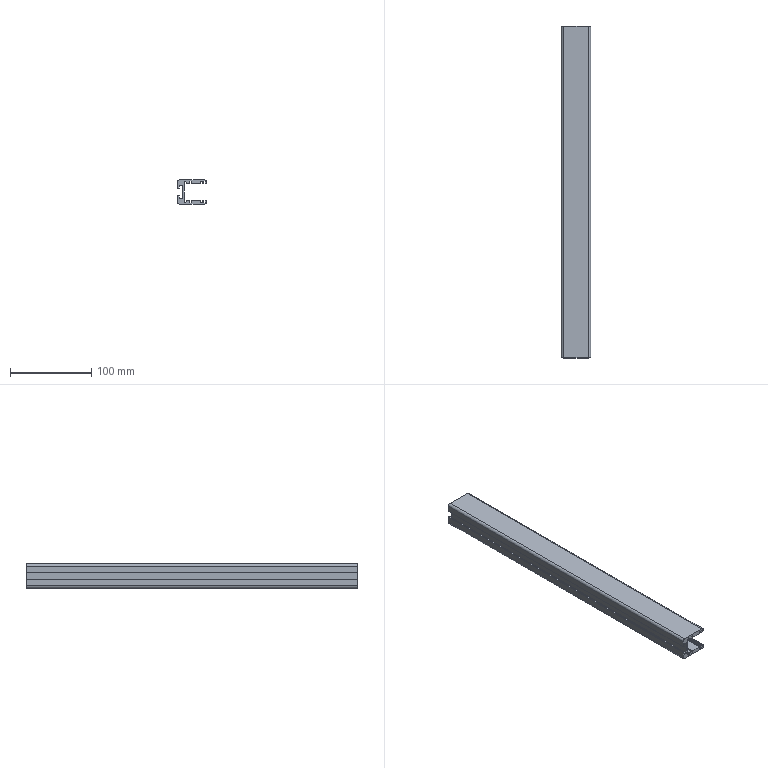Part | NX | 1 solid | 64 faces | box 36 x 409.7 x 30 mm | volume 154959 mm3 | plane 46 | cylinder 18 | commonest cylinder face diameters 0.4 x10 2.5 x4 6 x4